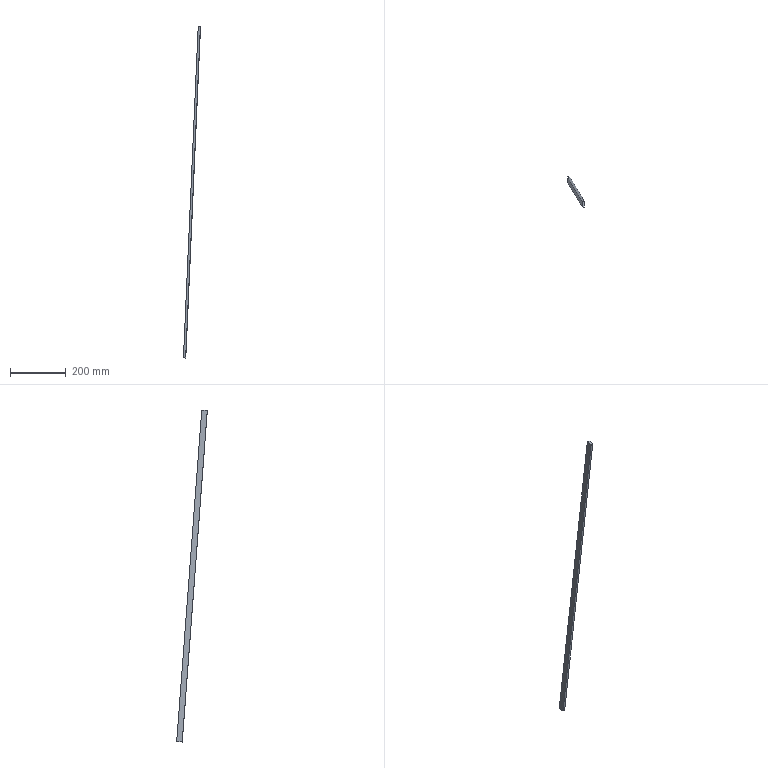Part | SolidWorks | features BaseBody 1 | 1 solid | 6 faces | box 61.56 x 110.498 x 1196 mm | volume 192110 mm3 | plane 6
STEP:
#1=CARTESIAN_POINT('',(-84.863,153.283,-1849.098));
#2=VERTEX_POINT('',#1);
#3=CARTESIAN_POINT('',(-92.852,153.492,-1848.727));
#4=VERTEX_POINT('',#3);
#5=CARTESIAN_POINT('',(-84.863,153.283,-1849.098));
#6=DIRECTION('',(-0.9986,0.0261,0.04626));
#7=VECTOR('',#6,1000.);
#8=LINE('',#5,#7);
#9=EDGE_CURVE('',#2,#4,#8,.T.);
#10=ORIENTED_EDGE('',*,*,#9,.F.);
#11=CARTESIAN_POINT('',(-85.387,133.235,-1849.098));
#12=VERTEX_POINT('',#11);
#13=CARTESIAN_POINT('',(-85.387,133.235,-1849.098));
#14=DIRECTION('',(0.02613,0.9997,0.));
#15=VECTOR('',#14,1000.);
#16=LINE('',#13,#15);
#17=EDGE_CURVE('',#12,#2,#16,.T.);
#18=ORIENTED_EDGE('',*,*,#17,.F.);
#19=CARTESIAN_POINT('',(-93.376,133.444,-1848.727));
#20=VERTEX_POINT('',#19);
#21=CARTESIAN_POINT('',(-93.376,133.444,-1848.727));
#22=DIRECTION('',(0.9986,-0.0261,-0.04626));
#23=VECTOR('',#22,1000.);
#24=LINE('',#21,#23);
#25=EDGE_CURVE('',#20,#12,#24,.T.);
#26=ORIENTED_EDGE('',*,*,#25,.F.);
#27=CARTESIAN_POINT('',(-92.852,153.492,-1848.727));
#28=DIRECTION('',(-0.02613,-0.9997,0.));
#29=VECTOR('',#28,1000.);
#30=LINE('',#27,#29);
#31=EDGE_CURVE('',#4,#20,#30,.T.);
#32=ORIENTED_EDGE('',*,*,#31,.F.);
#33=EDGE_LOOP('',(#10,#18,#26,#32));
#34=FACE_OUTER_BOUND('',#33,.T.);
#35=CARTESIAN_POINT('',(-84.812,153.613,-1849.099));
#36=DIRECTION('',(0.04624,-0.001208,0.9989));
#37=DIRECTION('',(-0.9989,0.,0.04624));
#38=AXIS2_PLACEMENT_3D('',#35,#36,#37);
#39=PLANE('',#38);
#40=ADVANCED_FACE('',(#34),#39,.F.);
#41=CARTESIAN_POINT('',(-40.329,43.202,-652.613));
#42=VERTEX_POINT('',#41);
#43=CARTESIAN_POINT('',(-40.329,43.202,-652.613));
#44=DIRECTION('',(-0.04418,0.07516,-0.9962));
#45=VECTOR('',#44,1000.);
#46=LINE('',#43,#45);
#47=EDGE_CURVE('',#42,#20,#46,.T.);
#48=ORIENTED_EDGE('',*,*,#47,.F.);
#49=CARTESIAN_POINT('',(-39.805,63.25,-652.613));
#50=VERTEX_POINT('',#49);
#51=CARTESIAN_POINT('',(-39.805,63.25,-652.613));
#52=DIRECTION('',(-0.02613,-0.9997,0.));
#53=VECTOR('',#52,1000.);
#54=LINE('',#51,#53);
#55=EDGE_CURVE('',#50,#42,#54,.T.);
#56=ORIENTED_EDGE('',*,*,#55,.F.);
#57=CARTESIAN_POINT('',(-92.852,153.492,-1848.727));
#58=DIRECTION('',(0.04418,-0.07516,0.9962));
#59=VECTOR('',#58,1000.);
#60=LINE('',#57,#59);
#61=EDGE_CURVE('',#4,#50,#60,.T.);
#62=ORIENTED_EDGE('',*,*,#61,.F.);
#63=ORIENTED_EDGE('',*,*,#31,.T.);
#64=EDGE_LOOP('',(#48,#56,#62,#63));
#65=FACE_OUTER_BOUND('',#64,.T.);
#66=CARTESIAN_POINT('',(-93.168,154.154,-1855.929));
#67=DIRECTION('',(0.9986,-0.0261,-0.04626));
#68=DIRECTION('',(0.04627,0.,0.9989));
#69=AXIS2_PLACEMENT_3D('',#66,#67,#68);
#70=PLANE('',#69);
#71=ADVANCED_FACE('',(#65),#70,.F.);
#72=CARTESIAN_POINT('',(-31.816,63.042,-652.983));
#73=VERTEX_POINT('',#72);
#74=CARTESIAN_POINT('',(-31.816,63.042,-652.983));
#75=DIRECTION('',(-0.9986,0.0261,0.04626));
#76=VECTOR('',#75,1000.);
#77=LINE('',#74,#76);
#78=EDGE_CURVE('',#73,#50,#77,.T.);
#79=ORIENTED_EDGE('',*,*,#78,.F.);
#80=CARTESIAN_POINT('',(-84.863,153.283,-1849.098));
#81=DIRECTION('',(0.04418,-0.07516,0.9962));
#82=VECTOR('',#81,1000.);
#83=LINE('',#80,#82);
#84=EDGE_CURVE('',#2,#73,#83,.T.);
#85=ORIENTED_EDGE('',*,*,#84,.F.);
#86=ORIENTED_EDGE('',*,*,#9,.T.);
#87=ORIENTED_EDGE('',*,*,#61,.T.);
#88=EDGE_LOOP('',(#79,#85,#86,#87));
#89=FACE_OUTER_BOUND('',#88,.T.);
#90=CARTESIAN_POINT('',(-31.45,152.245,-1856.393));
#91=DIRECTION('',(-0.02948,-0.9968,-0.0739));
#92=DIRECTION('',(0.,-0.07393,0.9973));
#93=AXIS2_PLACEMENT_3D('',#90,#91,#92);
#94=PLANE('',#93);
#95=ADVANCED_FACE('',(#89),#94,.F.);
#96=CARTESIAN_POINT('',(-32.34,42.994,-652.983));
#97=VERTEX_POINT('',#96);
#98=CARTESIAN_POINT('',(-31.816,63.042,-652.983));
#99=DIRECTION('',(-0.02613,-0.9997,-0.000000001));
#100=VECTOR('',#99,1000.);
#101=LINE('',#98,#100);
#102=EDGE_CURVE('',#73,#97,#101,.T.);
#103=ORIENTED_EDGE('',*,*,#102,.T.);
#104=CARTESIAN_POINT('',(-32.34,42.994,-652.983));
#105=DIRECTION('',(-0.04418,0.07516,-0.9962));
#106=VECTOR('',#105,1000.);
#107=LINE('',#104,#106);
#108=EDGE_CURVE('',#97,#12,#107,.T.);
#109=ORIENTED_EDGE('',*,*,#108,.T.);
#110=ORIENTED_EDGE('',*,*,#17,.T.);
#111=ORIENTED_EDGE('',*,*,#84,.T.);
#112=EDGE_LOOP('',(#103,#109,#110,#111));
#113=FACE_OUTER_BOUND('',#112,.T.);
#114=CARTESIAN_POINT('',(-85.179,153.945,-1856.299));
#115=DIRECTION('',(0.9986,-0.0261,-0.04626));
#116=DIRECTION('',(0.04627,0.,0.9989));
#117=AXIS2_PLACEMENT_3D('',#114,#115,#116);
#118=PLANE('',#117);
#119=ADVANCED_FACE('',(#113),#118,.T.);
#120=ORIENTED_EDGE('',*,*,#25,.T.);
#121=ORIENTED_EDGE('',*,*,#108,.F.);
#122=CARTESIAN_POINT('',(-40.329,43.202,-652.613));
#123=DIRECTION('',(0.9986,-0.0261,-0.04626));
#124=VECTOR('',#123,1000.);
#125=LINE('',#122,#124);
#126=EDGE_CURVE('',#42,#97,#125,.T.);
#127=ORIENTED_EDGE('',*,*,#126,.F.);
#128=ORIENTED_EDGE('',*,*,#47,.T.);
#129=EDGE_LOOP('',(#120,#121,#127,#128));
#130=FACE_OUTER_BOUND('',#129,.T.);
#131=CARTESIAN_POINT('',(-31.974,42.424,-645.452));
#132=DIRECTION('',(0.02948,0.9968,0.0739));
#133=DIRECTION('',(0.,0.07393,-0.9973));
#134=AXIS2_PLACEMENT_3D('',#131,#132,#133);
#135=PLANE('',#134);
#136=ADVANCED_FACE('',(#130),#135,.F.);
#137=ORIENTED_EDGE('',*,*,#126,.T.);
#138=ORIENTED_EDGE('',*,*,#102,.F.);
#139=ORIENTED_EDGE('',*,*,#78,.T.);
#140=ORIENTED_EDGE('',*,*,#55,.T.);
#141=EDGE_LOOP('',(#137,#138,#139,#140));
#142=FACE_OUTER_BOUND('',#141,.T.);
#143=CARTESIAN_POINT('',(-40.379,63.372,-652.586));
#144=DIRECTION('',(-0.04624,0.001208,-0.9989));
#145=DIRECTION('',(0.9989,0.,-0.04624));
#146=AXIS2_PLACEMENT_3D('',#143,#144,#145);
#147=PLANE('',#146);
#148=ADVANCED_FACE('',(#142),#147,.F.);
#149=CLOSED_SHELL('',(#40,#71,#95,#119,#136,#148));
#150=MANIFOLD_SOLID_BREP('',#149);
#151=CARTESIAN_POINT('',(0.,0.,0.));
#152=DIRECTION('',(0.,0.,1.));
#153=DIRECTION('',(1.,0.,0.));
#154=AXIS2_PLACEMENT_3D('',#151,#152,#153);
#155=(LENGTH_UNIT()NAMED_UNIT(*)SI_UNIT(.MILLI.,.METRE.));
#156=UNCERTAINTY_MEASURE_WITH_UNIT(LENGTH_MEASURE(0.00001),#155,'','');
#157=(NAMED_UNIT(*)PLANE_ANGLE_UNIT()SI_UNIT($,.RADIAN.));
#158=(NAMED_UNIT(*)SI_UNIT($,.STERADIAN.)SOLID_ANGLE_UNIT());
#159=(GEOMETRIC_REPRESENTATION_CONTEXT(3)GLOBAL_UNCERTAINTY_ASSIGNED_CONTEXT((#156))GLOBAL_UNIT_ASSIGNED_CONTEXT((#155,#157,#158))REPRESENTATION_CONTEXT('',''));
#160=ADVANCED_BREP_SHAPE_REPRESENTATION('',(#150,#154),#159);